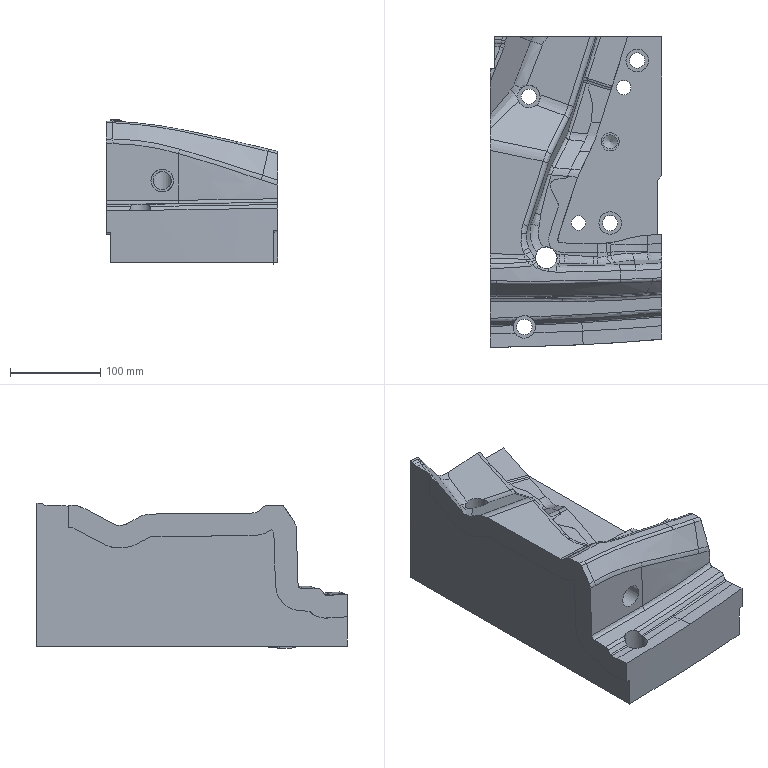Part | NX | features solid 2 | 1 solid | 160 faces | box 190.002 x 344.132 x 158.004 mm | volume 5737401 mm3 | spline 128 | plane 15 | cylinder 15 | sphere 1 | cone 1 | commonest cylinder face diameters 25 x5 17 x4 16 x3 20 x2 24 x1